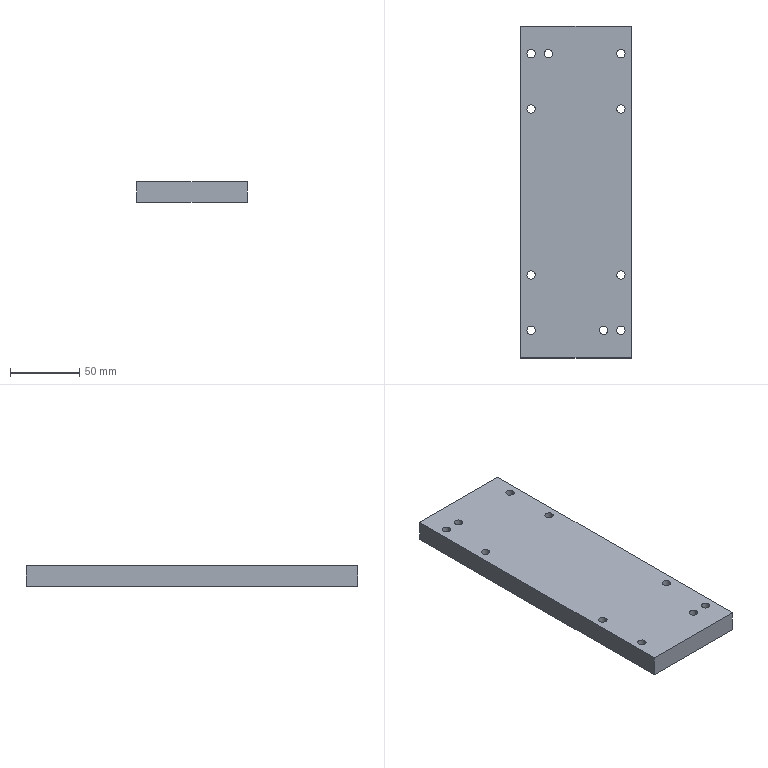Part | STEP file | SN10_008_006-02_PLACA | 1 solid | 16 faces | box 80 x 240 x 15 mm | volume 283759 mm3 | cylinder 10 | plane 6 | commonest cylinder face diameters 6 x10
STEP:
#1=CARTESIAN_POINT('',(0.,0.,0.));
#2=DIRECTION('',(0.,0.,1.));
#3=DIRECTION('',(1.,0.,0.));
#4=AXIS2_PLACEMENT_3D('',#1,#2,#3);
#5=CARTESIAN_POINT('',(323.629,430.,-115.));
#6=VERTEX_POINT('',#5);
#7=CARTESIAN_POINT('',(323.629,190.,-115.));
#8=VERTEX_POINT('',#7);
#9=CARTESIAN_POINT('',(323.629,430.,-115.));
#10=DIRECTION('',(0.,-1.,0.));
#11=VECTOR('',#10,1.);
#12=LINE('',#9,#11);
#13=CARTESIAN_POINT('',(0.,0.,-115.));
#14=DIRECTION('',(0.,0.,1.));
#15=DIRECTION('',(1.,0.,0.));
#16=AXIS2_PLACEMENT_3D('',#13,#14,#15);
#17=PLANE('',#16);
#18=CARTESIAN_POINT('',(323.629,430.));
#19=DIRECTION('',(0.,-1.));
#20=VECTOR('',#19,1.);
#21=LINE('',#18,#20);
#22=(GEOMETRIC_REPRESENTATION_CONTEXT(2)PARAMETRIC_REPRESENTATION_CONTEXT()REPRESENTATION_CONTEXT('',''));
#23=DEFINITIONAL_REPRESENTATION('',(#21),#22);
#24=PCURVE('',#17,#23);
#25=CARTESIAN_POINT('',(323.629,430.,-115.));
#26=DIRECTION('',(-1.,0.,0.));
#27=DIRECTION('',(0.,0.,1.));
#28=AXIS2_PLACEMENT_3D('',#25,#26,#27);
#29=PLANE('',#28);
#30=CARTESIAN_POINT('',(0.,0.));
#31=DIRECTION('',(0.,-1.));
#32=VECTOR('',#31,1.);
#33=LINE('',#30,#32);
#34=(GEOMETRIC_REPRESENTATION_CONTEXT(2)PARAMETRIC_REPRESENTATION_CONTEXT()REPRESENTATION_CONTEXT('',''));
#35=DEFINITIONAL_REPRESENTATION('',(#33),#34);
#36=PCURVE('',#29,#35);
#37=SURFACE_CURVE('',#12,(#24,#36),.PCURVE_S1.);
#38=EDGE_CURVE('',#6,#8,#37,.T.);
#39=ORIENTED_EDGE('',*,*,#38,.T.);
#40=CARTESIAN_POINT('',(243.629,190.,-115.));
#41=VERTEX_POINT('',#40);
#42=CARTESIAN_POINT('',(323.629,190.,-115.));
#43=DIRECTION('',(-1.,0.,0.));
#44=VECTOR('',#43,1.);
#45=LINE('',#42,#44);
#46=CARTESIAN_POINT('',(323.629,190.));
#47=DIRECTION('',(-1.,0.));
#48=VECTOR('',#47,1.);
#49=LINE('',#46,#48);
#50=(GEOMETRIC_REPRESENTATION_CONTEXT(2)PARAMETRIC_REPRESENTATION_CONTEXT()REPRESENTATION_CONTEXT('',''));
#51=DEFINITIONAL_REPRESENTATION('',(#49),#50);
#52=PCURVE('',#17,#51);
#53=CARTESIAN_POINT('',(323.629,190.,-115.));
#54=DIRECTION('',(0.,1.,0.));
#55=DIRECTION('',(0.,0.,1.));
#56=AXIS2_PLACEMENT_3D('',#53,#54,#55);
#57=PLANE('',#56);
#58=CARTESIAN_POINT('',(0.,0.));
#59=DIRECTION('',(0.,-1.));
#60=VECTOR('',#59,1.);
#61=LINE('',#58,#60);
#62=(GEOMETRIC_REPRESENTATION_CONTEXT(2)PARAMETRIC_REPRESENTATION_CONTEXT()REPRESENTATION_CONTEXT('',''));
#63=DEFINITIONAL_REPRESENTATION('',(#61),#62);
#64=PCURVE('',#57,#63);
#65=SURFACE_CURVE('',#45,(#52,#64),.PCURVE_S1.);
#66=EDGE_CURVE('',#8,#41,#65,.T.);
#67=ORIENTED_EDGE('',*,*,#66,.T.);
#68=CARTESIAN_POINT('',(243.629,430.,-115.));
#69=VERTEX_POINT('',#68);
#70=CARTESIAN_POINT('',(243.629,190.,-115.));
#71=DIRECTION('',(0.,1.,0.));
#72=VECTOR('',#71,1.);
#73=LINE('',#70,#72);
#74=CARTESIAN_POINT('',(243.629,190.));
#75=DIRECTION('',(0.,1.));
#76=VECTOR('',#75,1.);
#77=LINE('',#74,#76);
#78=(GEOMETRIC_REPRESENTATION_CONTEXT(2)PARAMETRIC_REPRESENTATION_CONTEXT()REPRESENTATION_CONTEXT('',''));
#79=DEFINITIONAL_REPRESENTATION('',(#77),#78);
#80=PCURVE('',#17,#79);
#81=CARTESIAN_POINT('',(243.629,190.,-115.));
#82=DIRECTION('',(1.,0.,0.));
#83=DIRECTION('',(0.,0.,-1.));
#84=AXIS2_PLACEMENT_3D('',#81,#82,#83);
#85=PLANE('',#84);
#86=CARTESIAN_POINT('',(0.,0.));
#87=DIRECTION('',(0.,1.));
#88=VECTOR('',#87,1.);
#89=LINE('',#86,#88);
#90=(GEOMETRIC_REPRESENTATION_CONTEXT(2)PARAMETRIC_REPRESENTATION_CONTEXT()REPRESENTATION_CONTEXT('',''));
#91=DEFINITIONAL_REPRESENTATION('',(#89),#90);
#92=PCURVE('',#85,#91);
#93=SURFACE_CURVE('',#73,(#80,#92),.PCURVE_S1.);
#94=EDGE_CURVE('',#41,#69,#93,.T.);
#95=ORIENTED_EDGE('',*,*,#94,.T.);
#96=CARTESIAN_POINT('',(243.629,430.,-115.));
#97=DIRECTION('',(1.,0.,0.));
#98=VECTOR('',#97,1.);
#99=LINE('',#96,#98);
#100=CARTESIAN_POINT('',(243.629,430.));
#101=DIRECTION('',(1.,0.));
#102=VECTOR('',#101,1.);
#103=LINE('',#100,#102);
#104=(GEOMETRIC_REPRESENTATION_CONTEXT(2)PARAMETRIC_REPRESENTATION_CONTEXT()REPRESENTATION_CONTEXT('',''));
#105=DEFINITIONAL_REPRESENTATION('',(#103),#104);
#106=PCURVE('',#17,#105);
#107=CARTESIAN_POINT('',(243.629,430.,-115.));
#108=DIRECTION('',(0.,-1.,0.));
#109=DIRECTION('',(0.,0.,-1.));
#110=AXIS2_PLACEMENT_3D('',#107,#108,#109);
#111=PLANE('',#110);
#112=CARTESIAN_POINT('',(0.,0.));
#113=DIRECTION('',(0.,1.));
#114=VECTOR('',#113,1.);
#115=LINE('',#112,#114);
#116=(GEOMETRIC_REPRESENTATION_CONTEXT(2)PARAMETRIC_REPRESENTATION_CONTEXT()REPRESENTATION_CONTEXT('',''));
#117=DEFINITIONAL_REPRESENTATION('',(#115),#116);
#118=PCURVE('',#111,#117);
#119=SURFACE_CURVE('',#99,(#106,#118),.PCURVE_S1.);
#120=EDGE_CURVE('',#69,#6,#119,.T.);
#121=ORIENTED_EDGE('',*,*,#120,.T.);
#122=EDGE_LOOP('',(#39,#67,#95,#121));
#123=FACE_BOUND('',#122,.T.);
#124=CARTESIAN_POINT('',(318.762,211.438,-115.));
#125=VERTEX_POINT('',#124);
#126=CARTESIAN_POINT('',(316.129,210.,-115.));
#127=DIRECTION('',(0.,0.,1.));
#128=DIRECTION('',(1.,0.,0.));
#129=AXIS2_PLACEMENT_3D('',#126,#127,#128);
#130=CIRCLE('',#129,3.);
#131=CARTESIAN_POINT('',(316.129,210.));
#132=DIRECTION('',(1.,0.));
#133=AXIS2_PLACEMENT_2D('',#131,#132);
#134=CIRCLE('',#133,3.);
#135=(GEOMETRIC_REPRESENTATION_CONTEXT(2)PARAMETRIC_REPRESENTATION_CONTEXT()REPRESENTATION_CONTEXT('',''));
#136=DEFINITIONAL_REPRESENTATION('',(#134),#135);
#137=PCURVE('',#17,#136);
#138=CARTESIAN_POINT('',(316.129,210.,-114.9));
#139=DIRECTION('',(0.,0.,1.));
#140=DIRECTION('',(0.8776,0.4794,0.));
#141=AXIS2_PLACEMENT_3D('',#138,#139,#140);
#142=CYLINDRICAL_SURFACE('',#141,3.);
#143=CARTESIAN_POINT('',(-0.5,-0.1));
#144=DIRECTION('',(1.,0.));
#145=VECTOR('',#144,1.);
#146=LINE('',#143,#145);
#147=(GEOMETRIC_REPRESENTATION_CONTEXT(2)PARAMETRIC_REPRESENTATION_CONTEXT()REPRESENTATION_CONTEXT('',''));
#148=DEFINITIONAL_REPRESENTATION('',(#146),#147);
#149=PCURVE('',#142,#148);
#150=SURFACE_CURVE('',#130,(#137,#149),.PCURVE_S1.);
#151=EDGE_CURVE('',#125,#125,#150,.T.);
#152=ORIENTED_EDGE('',*,*,#151,.T.);
#153=EDGE_LOOP('',(#152));
#154=FACE_BOUND('',#153,.T.);
#155=CARTESIAN_POINT('',(253.762,411.438,-115.));
#156=VERTEX_POINT('',#155);
#157=CARTESIAN_POINT('',(251.129,410.,-115.));
#158=DIRECTION('',(0.,0.,1.));
#159=DIRECTION('',(1.,0.,0.));
#160=AXIS2_PLACEMENT_3D('',#157,#158,#159);
#161=CIRCLE('',#160,3.);
#162=CARTESIAN_POINT('',(251.129,410.));
#163=DIRECTION('',(1.,0.));
#164=AXIS2_PLACEMENT_2D('',#162,#163);
#165=CIRCLE('',#164,3.);
#166=(GEOMETRIC_REPRESENTATION_CONTEXT(2)PARAMETRIC_REPRESENTATION_CONTEXT()REPRESENTATION_CONTEXT('',''));
#167=DEFINITIONAL_REPRESENTATION('',(#165),#166);
#168=PCURVE('',#17,#167);
#169=CARTESIAN_POINT('',(251.129,410.,-114.9));
#170=DIRECTION('',(0.,0.,1.));
#171=DIRECTION('',(0.8776,0.4794,0.));
#172=AXIS2_PLACEMENT_3D('',#169,#170,#171);
#173=CYLINDRICAL_SURFACE('',#172,3.);
#174=CARTESIAN_POINT('',(-0.5,-0.1));
#175=DIRECTION('',(1.,0.));
#176=VECTOR('',#175,1.);
#177=LINE('',#174,#176);
#178=(GEOMETRIC_REPRESENTATION_CONTEXT(2)PARAMETRIC_REPRESENTATION_CONTEXT()REPRESENTATION_CONTEXT('',''));
#179=DEFINITIONAL_REPRESENTATION('',(#177),#178);
#180=PCURVE('',#173,#179);
#181=SURFACE_CURVE('',#161,(#168,#180),.PCURVE_S1.);
#182=EDGE_CURVE('',#156,#156,#181,.T.);
#183=ORIENTED_EDGE('',*,*,#182,.T.);
#184=EDGE_LOOP('',(#183));
#185=FACE_BOUND('',#184,.T.);
#186=CARTESIAN_POINT('',(306.262,211.438,-115.));
#187=VERTEX_POINT('',#186);
#188=CARTESIAN_POINT('',(303.629,210.,-115.));
#189=DIRECTION('',(0.,0.,1.));
#190=DIRECTION('',(1.,0.,0.));
#191=AXIS2_PLACEMENT_3D('',#188,#189,#190);
#192=CIRCLE('',#191,3.);
#193=CARTESIAN_POINT('',(303.629,210.));
#194=DIRECTION('',(1.,0.));
#195=AXIS2_PLACEMENT_2D('',#193,#194);
#196=CIRCLE('',#195,3.);
#197=(GEOMETRIC_REPRESENTATION_CONTEXT(2)PARAMETRIC_REPRESENTATION_CONTEXT()REPRESENTATION_CONTEXT('',''));
#198=DEFINITIONAL_REPRESENTATION('',(#196),#197);
#199=PCURVE('',#17,#198);
#200=CARTESIAN_POINT('',(303.629,210.,-114.9));
#201=DIRECTION('',(0.,0.,1.));
#202=DIRECTION('',(0.8776,0.4794,0.));
#203=AXIS2_PLACEMENT_3D('',#200,#201,#202);
#204=CYLINDRICAL_SURFACE('',#203,3.);
#205=CARTESIAN_POINT('',(-0.5,-0.1));
#206=DIRECTION('',(1.,0.));
#207=VECTOR('',#206,1.);
#208=LINE('',#205,#207);
#209=(GEOMETRIC_REPRESENTATION_CONTEXT(2)PARAMETRIC_REPRESENTATION_CONTEXT()REPRESENTATION_CONTEXT('',''));
#210=DEFINITIONAL_REPRESENTATION('',(#208),#209);
#211=PCURVE('',#204,#210);
#212=SURFACE_CURVE('',#192,(#199,#211),.PCURVE_S1.);
#213=EDGE_CURVE('',#187,#187,#212,.T.);
#214=ORIENTED_EDGE('',*,*,#213,.T.);
#215=EDGE_LOOP('',(#214));
#216=FACE_BOUND('',#215,.T.);
#217=CARTESIAN_POINT('',(266.262,411.438,-115.));
#218=VERTEX_POINT('',#217);
#219=CARTESIAN_POINT('',(263.629,410.,-115.));
#220=DIRECTION('',(0.,0.,1.));
#221=DIRECTION('',(1.,0.,0.));
#222=AXIS2_PLACEMENT_3D('',#219,#220,#221);
#223=CIRCLE('',#222,3.);
#224=CARTESIAN_POINT('',(263.629,410.));
#225=DIRECTION('',(1.,0.));
#226=AXIS2_PLACEMENT_2D('',#224,#225);
#227=CIRCLE('',#226,3.);
#228=(GEOMETRIC_REPRESENTATION_CONTEXT(2)PARAMETRIC_REPRESENTATION_CONTEXT()REPRESENTATION_CONTEXT('',''));
#229=DEFINITIONAL_REPRESENTATION('',(#227),#228);
#230=PCURVE('',#17,#229);
#231=CARTESIAN_POINT('',(263.629,410.,-114.9));
#232=DIRECTION('',(0.,0.,1.));
#233=DIRECTION('',(0.8776,0.4794,0.));
#234=AXIS2_PLACEMENT_3D('',#231,#232,#233);
#235=CYLINDRICAL_SURFACE('',#234,3.);
#236=CARTESIAN_POINT('',(-0.5,-0.1));
#237=DIRECTION('',(1.,0.));
#238=VECTOR('',#237,1.);
#239=LINE('',#236,#238);
#240=(GEOMETRIC_REPRESENTATION_CONTEXT(2)PARAMETRIC_REPRESENTATION_CONTEXT()REPRESENTATION_CONTEXT('',''));
#241=DEFINITIONAL_REPRESENTATION('',(#239),#240);
#242=PCURVE('',#235,#241);
#243=SURFACE_CURVE('',#223,(#230,#242),.PCURVE_S1.);
#244=EDGE_CURVE('',#218,#218,#243,.T.);
#245=ORIENTED_EDGE('',*,*,#244,.T.);
#246=EDGE_LOOP('',(#245));
#247=FACE_BOUND('',#246,.T.);
#248=CARTESIAN_POINT('',(313.496,408.562,-115.));
#249=VERTEX_POINT('',#248);
#250=CARTESIAN_POINT('',(316.129,410.,-115.));
#251=DIRECTION('',(0.,0.,1.));
#252=DIRECTION('',(1.,0.,0.));
#253=AXIS2_PLACEMENT_3D('',#250,#251,#252);
#254=CIRCLE('',#253,3.);
#255=CARTESIAN_POINT('',(316.129,410.));
#256=DIRECTION('',(1.,0.));
#257=AXIS2_PLACEMENT_2D('',#255,#256);
#258=CIRCLE('',#257,3.);
#259=(GEOMETRIC_REPRESENTATION_CONTEXT(2)PARAMETRIC_REPRESENTATION_CONTEXT()REPRESENTATION_CONTEXT('',''));
#260=DEFINITIONAL_REPRESENTATION('',(#258),#259);
#261=PCURVE('',#17,#260);
#262=CARTESIAN_POINT('',(316.129,410.,-114.9));
#263=DIRECTION('',(0.,0.,1.));
#264=DIRECTION('',(0.8776,0.4794,0.));
#265=AXIS2_PLACEMENT_3D('',#262,#263,#264);
#266=CYLINDRICAL_SURFACE('',#265,3.);
#267=CARTESIAN_POINT('',(-0.5,-0.1));
#268=DIRECTION('',(1.,0.));
#269=VECTOR('',#268,1.);
#270=LINE('',#267,#269);
#271=(GEOMETRIC_REPRESENTATION_CONTEXT(2)PARAMETRIC_REPRESENTATION_CONTEXT()REPRESENTATION_CONTEXT('',''));
#272=DEFINITIONAL_REPRESENTATION('',(#270),#271);
#273=PCURVE('',#266,#272);
#274=SURFACE_CURVE('',#254,(#261,#273),.PCURVE_S1.);
#275=EDGE_CURVE('',#249,#249,#274,.T.);
#276=ORIENTED_EDGE('',*,*,#275,.T.);
#277=EDGE_LOOP('',(#276));
#278=FACE_BOUND('',#277,.T.);
#279=CARTESIAN_POINT('',(248.496,368.562,-115.));
#280=VERTEX_POINT('',#279);
#281=CARTESIAN_POINT('',(251.129,370.,-115.));
#282=DIRECTION('',(0.,0.,1.));
#283=DIRECTION('',(1.,0.,0.));
#284=AXIS2_PLACEMENT_3D('',#281,#282,#283);
#285=CIRCLE('',#284,3.);
#286=CARTESIAN_POINT('',(251.129,370.));
#287=DIRECTION('',(1.,0.));
#288=AXIS2_PLACEMENT_2D('',#286,#287);
#289=CIRCLE('',#288,3.);
#290=(GEOMETRIC_REPRESENTATION_CONTEXT(2)PARAMETRIC_REPRESENTATION_CONTEXT()REPRESENTATION_CONTEXT('',''));
#291=DEFINITIONAL_REPRESENTATION('',(#289),#290);
#292=PCURVE('',#17,#291);
#293=CARTESIAN_POINT('',(251.129,370.,-114.9));
#294=DIRECTION('',(0.,0.,1.));
#295=DIRECTION('',(0.8776,0.4794,0.));
#296=AXIS2_PLACEMENT_3D('',#293,#294,#295);
#297=CYLINDRICAL_SURFACE('',#296,3.);
#298=CARTESIAN_POINT('',(-0.5,-0.1));
#299=DIRECTION('',(1.,0.));
#300=VECTOR('',#299,1.);
#301=LINE('',#298,#300);
#302=(GEOMETRIC_REPRESENTATION_CONTEXT(2)PARAMETRIC_REPRESENTATION_CONTEXT()REPRESENTATION_CONTEXT('',''));
#303=DEFINITIONAL_REPRESENTATION('',(#301),#302);
#304=PCURVE('',#297,#303);
#305=SURFACE_CURVE('',#285,(#292,#304),.PCURVE_S1.);
#306=EDGE_CURVE('',#280,#280,#305,.T.);
#307=ORIENTED_EDGE('',*,*,#306,.T.);
#308=EDGE_LOOP('',(#307));
#309=FACE_BOUND('',#308,.T.);
#310=CARTESIAN_POINT('',(313.496,368.562,-115.));
#311=VERTEX_POINT('',#310);
#312=CARTESIAN_POINT('',(316.129,370.,-115.));
#313=DIRECTION('',(0.,0.,1.));
#314=DIRECTION('',(1.,0.,0.));
#315=AXIS2_PLACEMENT_3D('',#312,#313,#314);
#316=CIRCLE('',#315,3.);
#317=CARTESIAN_POINT('',(316.129,370.));
#318=DIRECTION('',(1.,0.));
#319=AXIS2_PLACEMENT_2D('',#317,#318);
#320=CIRCLE('',#319,3.);
#321=(GEOMETRIC_REPRESENTATION_CONTEXT(2)PARAMETRIC_REPRESENTATION_CONTEXT()REPRESENTATION_CONTEXT('',''));
#322=DEFINITIONAL_REPRESENTATION('',(#320),#321);
#323=PCURVE('',#17,#322);
#324=CARTESIAN_POINT('',(316.129,370.,-114.9));
#325=DIRECTION('',(0.,0.,1.));
#326=DIRECTION('',(0.8776,0.4794,0.));
#327=AXIS2_PLACEMENT_3D('',#324,#325,#326);
#328=CYLINDRICAL_SURFACE('',#327,3.);
#329=CARTESIAN_POINT('',(-0.5,-0.1));
#330=DIRECTION('',(1.,0.));
#331=VECTOR('',#330,1.);
#332=LINE('',#329,#331);
#333=(GEOMETRIC_REPRESENTATION_CONTEXT(2)PARAMETRIC_REPRESENTATION_CONTEXT()REPRESENTATION_CONTEXT('',''));
#334=DEFINITIONAL_REPRESENTATION('',(#332),#333);
#335=PCURVE('',#328,#334);
#336=SURFACE_CURVE('',#316,(#323,#335),.PCURVE_S1.);
#337=EDGE_CURVE('',#311,#311,#336,.T.);
#338=ORIENTED_EDGE('',*,*,#337,.T.);
#339=EDGE_LOOP('',(#338));
#340=FACE_BOUND('',#339,.T.);
#341=CARTESIAN_POINT('',(253.762,211.438,-115.));
#342=VERTEX_POINT('',#341);
#343=CARTESIAN_POINT('',(251.129,210.,-115.));
#344=DIRECTION('',(0.,0.,1.));
#345=DIRECTION('',(1.,0.,0.));
#346=AXIS2_PLACEMENT_3D('',#343,#344,#345);
#347=CIRCLE('',#346,3.);
#348=CARTESIAN_POINT('',(251.129,210.));
#349=DIRECTION('',(1.,0.));
#350=AXIS2_PLACEMENT_2D('',#348,#349);
#351=CIRCLE('',#350,3.);
#352=(GEOMETRIC_REPRESENTATION_CONTEXT(2)PARAMETRIC_REPRESENTATION_CONTEXT()REPRESENTATION_CONTEXT('',''));
#353=DEFINITIONAL_REPRESENTATION('',(#351),#352);
#354=PCURVE('',#17,#353);
#355=CARTESIAN_POINT('',(251.129,210.,-114.9));
#356=DIRECTION('',(0.,0.,1.));
#357=DIRECTION('',(0.8776,0.4794,0.));
#358=AXIS2_PLACEMENT_3D('',#355,#356,#357);
#359=CYLINDRICAL_SURFACE('',#358,3.);
#360=CARTESIAN_POINT('',(-0.5,-0.1));
#361=DIRECTION('',(1.,0.));
#362=VECTOR('',#361,1.);
#363=LINE('',#360,#362);
#364=(GEOMETRIC_REPRESENTATION_CONTEXT(2)PARAMETRIC_REPRESENTATION_CONTEXT()REPRESENTATION_CONTEXT('',''));
#365=DEFINITIONAL_REPRESENTATION('',(#363),#364);
#366=PCURVE('',#359,#365);
#367=SURFACE_CURVE('',#347,(#354,#366),.PCURVE_S1.);
#368=EDGE_CURVE('',#342,#342,#367,.T.);
#369=ORIENTED_EDGE('',*,*,#368,.T.);
#370=EDGE_LOOP('',(#369));
#371=FACE_BOUND('',#370,.T.);
#372=CARTESIAN_POINT('',(318.762,251.438,-115.));
#373=VERTEX_POINT('',#372);
#374=CARTESIAN_POINT('',(316.129,250.,-115.));
#375=DIRECTION('',(0.,0.,1.));
#376=DIRECTION('',(1.,0.,0.));
#377=AXIS2_PLACEMENT_3D('',#374,#375,#376);
#378=CIRCLE('',#377,3.);
#379=CARTESIAN_POINT('',(316.129,250.));
#380=DIRECTION('',(1.,0.));
#381=AXIS2_PLACEMENT_2D('',#379,#380);
#382=CIRCLE('',#381,3.);
#383=(GEOMETRIC_REPRESENTATION_CONTEXT(2)PARAMETRIC_REPRESENTATION_CONTEXT()REPRESENTATION_CONTEXT('',''));
#384=DEFINITIONAL_REPRESENTATION('',(#382),#383);
#385=PCURVE('',#17,#384);
#386=CARTESIAN_POINT('',(316.129,250.,-114.9));
#387=DIRECTION('',(0.,0.,1.));
#388=DIRECTION('',(0.8776,0.4794,0.));
#389=AXIS2_PLACEMENT_3D('',#386,#387,#388);
#390=CYLINDRICAL_SURFACE('',#389,3.);
#391=CARTESIAN_POINT('',(-0.5,-0.1));
#392=DIRECTION('',(1.,0.));
#393=VECTOR('',#392,1.);
#394=LINE('',#391,#393);
#395=(GEOMETRIC_REPRESENTATION_CONTEXT(2)PARAMETRIC_REPRESENTATION_CONTEXT()REPRESENTATION_CONTEXT('',''));
#396=DEFINITIONAL_REPRESENTATION('',(#394),#395);
#397=PCURVE('',#390,#396);
#398=SURFACE_CURVE('',#378,(#385,#397),.PCURVE_S1.);
#399=EDGE_CURVE('',#373,#373,#398,.T.);
#400=ORIENTED_EDGE('',*,*,#399,.T.);
#401=EDGE_LOOP('',(#400));
#402=FACE_BOUND('',#401,.T.);
#403=CARTESIAN_POINT('',(253.762,251.438,-115.));
#404=VERTEX_POINT('',#403);
#405=CARTESIAN_POINT('',(251.129,250.,-115.));
#406=DIRECTION('',(0.,0.,1.));
#407=DIRECTION('',(1.,0.,0.));
#408=AXIS2_PLACEMENT_3D('',#405,#406,#407);
#409=CIRCLE('',#408,3.);
#410=CARTESIAN_POINT('',(251.129,250.));
#411=DIRECTION('',(1.,0.));
#412=AXIS2_PLACEMENT_2D('',#410,#411);
#413=CIRCLE('',#412,3.);
#414=(GEOMETRIC_REPRESENTATION_CONTEXT(2)PARAMETRIC_REPRESENTATION_CONTEXT()REPRESENTATION_CONTEXT('',''));
#415=DEFINITIONAL_REPRESENTATION('',(#413),#414);
#416=PCURVE('',#17,#415);
#417=CARTESIAN_POINT('',(251.129,250.,-114.9));
#418=DIRECTION('',(0.,0.,1.));
#419=DIRECTION('',(0.8776,0.4794,0.));
#420=AXIS2_PLACEMENT_3D('',#417,#418,#419);
#421=CYLINDRICAL_SURFACE('',#420,3.);
#422=CARTESIAN_POINT('',(-0.5,-0.1));
#423=DIRECTION('',(1.,0.));
#424=VECTOR('',#423,1.);
#425=LINE('',#422,#424);
#426=(GEOMETRIC_REPRESENTATION_CONTEXT(2)PARAMETRIC_REPRESENTATION_CONTEXT()REPRESENTATION_CONTEXT('',''));
#427=DEFINITIONAL_REPRESENTATION('',(#425),#426);
#428=PCURVE('',#421,#427);
#429=SURFACE_CURVE('',#409,(#416,#428),.PCURVE_S1.);
#430=EDGE_CURVE('',#404,#404,#429,.T.);
#431=ORIENTED_EDGE('',*,*,#430,.T.);
#432=EDGE_LOOP('',(#431));
#433=FACE_BOUND('',#432,.T.);
#434=ADVANCED_FACE('',(#123,#154,#185,#216,#247,#278,#309,#340,#371,#402,#433),#17,.F.);
#435=CARTESIAN_POINT('',(253.762,211.438,-100.));
#436=VERTEX_POINT('',#435);
#437=CARTESIAN_POINT('',(251.129,210.,-100.));
#438=DIRECTION('',(0.,0.,1.));
#439=DIRECTION('',(1.,0.,0.));
#440=AXIS2_PLACEMENT_3D('',#437,#438,#439);
#441=CIRCLE('',#440,3.);
#442=CARTESIAN_POINT('',(-0.5,14.9));
#443=DIRECTION('',(1.,0.));
#444=VECTOR('',#443,1.);
#445=LINE('',#442,#444);
#446=(GEOMETRIC_REPRESENTATION_CONTEXT(2)PARAMETRIC_REPRESENTATION_CONTEXT()REPRESENTATION_CONTEXT('',''));
#447=DEFINITIONAL_REPRESENTATION('',(#445),#446);
#448=PCURVE('',#359,#447);
#449=CARTESIAN_POINT('',(0.,0.,-100.));
#450=DIRECTION('',(0.,0.,1.));
#451=DIRECTION('',(1.,0.,0.));
#452=AXIS2_PLACEMENT_3D('',#449,#450,#451);
#453=PLANE('',#452);
#454=CARTESIAN_POINT('',(251.129,210.));
#455=DIRECTION('',(1.,0.));
#456=AXIS2_PLACEMENT_2D('',#454,#455);
#457=CIRCLE('',#456,3.);
#458=(GEOMETRIC_REPRESENTATION_CONTEXT(2)PARAMETRIC_REPRESENTATION_CONTEXT()REPRESENTATION_CONTEXT('',''));
#459=DEFINITIONAL_REPRESENTATION('',(#457),#458);
#460=PCURVE('',#453,#459);
#461=SURFACE_CURVE('',#441,(#448,#460),.PCURVE_S1.);
#462=EDGE_CURVE('',#436,#436,#461,.T.);
#463=ORIENTED_EDGE('',*,*,#462,.F.);
#464=CARTESIAN_POINT('',(253.762,211.438,-115.));
#465=CARTESIAN_POINT('',(253.762,211.438,-100.));
#466=B_SPLINE_CURVE_WITH_KNOTS('',1,(#464,#465),.UNSPECIFIED.,.F.,.F.,(2,2),(-0.1,14.9),.PIECEWISE_BEZIER_KNOTS.);
#467=CARTESIAN_POINT('',(0.,0.));
#468=DIRECTION('',(0.,1.));
#469=VECTOR('',#468,1.);
#470=LINE('',#467,#469);
#471=(GEOMETRIC_REPRESENTATION_CONTEXT(2)PARAMETRIC_REPRESENTATION_CONTEXT()REPRESENTATION_CONTEXT('',''));
#472=DEFINITIONAL_REPRESENTATION('',(#470),#471);
#473=PCURVE('',#359,#472);
#474=CARTESIAN_POINT('',(6.283,0.));
#475=DIRECTION('',(0.,1.));
#476=VECTOR('',#475,1.);
#477=LINE('',#474,#476);
#478=(GEOMETRIC_REPRESENTATION_CONTEXT(2)PARAMETRIC_REPRESENTATION_CONTEXT()REPRESENTATION_CONTEXT('',''));
#479=DEFINITIONAL_REPRESENTATION('',(#477),#478);
#480=PCURVE('',#359,#479);
#481=SEAM_CURVE('',#466,(#473,#480),.PCURVE_S1.);
#482=EDGE_CURVE('',#342,#436,#481,.T.);
#483=ORIENTED_EDGE('',*,*,#482,.F.);
#484=ORIENTED_EDGE('',*,*,#368,.T.);
#485=ORIENTED_EDGE('',*,*,#482,.T.);
#486=EDGE_LOOP('',(#463,#483,#484,#485));
#487=FACE_BOUND('',#486,.F.);
#488=ADVANCED_FACE('',(#487),#359,.F.);
#489=CARTESIAN_POINT('',(318.762,251.438,-100.));
#490=VERTEX_POINT('',#489);
#491=CARTESIAN_POINT('',(316.129,250.,-100.));
#492=DIRECTION('',(0.,0.,1.));
#493=DIRECTION('',(1.,0.,0.));
#494=AXIS2_PLACEMENT_3D('',#491,#492,#493);
#495=CIRCLE('',#494,3.);
#496=CARTESIAN_POINT('',(-0.5,14.9));
#497=DIRECTION('',(1.,0.));
#498=VECTOR('',#497,1.);
#499=LINE('',#496,#498);
#500=(GEOMETRIC_REPRESENTATION_CONTEXT(2)PARAMETRIC_REPRESENTATION_CONTEXT()REPRESENTATION_CONTEXT('',''));
#501=DEFINITIONAL_REPRESENTATION('',(#499),#500);
#502=PCURVE('',#390,#501);
#503=CARTESIAN_POINT('',(316.129,250.));
#504=DIRECTION('',(1.,0.));
#505=AXIS2_PLACEMENT_2D('',#503,#504);
#506=CIRCLE('',#505,3.);
#507=(GEOMETRIC_REPRESENTATION_CONTEXT(2)PARAMETRIC_REPRESENTATION_CONTEXT()REPRESENTATION_CONTEXT('',''));
#508=DEFINITIONAL_REPRESENTATION('',(#506),#507);
#509=PCURVE('',#453,#508);
#510=SURFACE_CURVE('',#495,(#502,#509),.PCURVE_S1.);
#511=EDGE_CURVE('',#490,#490,#510,.T.);
#512=ORIENTED_EDGE('',*,*,#511,.F.);
#513=CARTESIAN_POINT('',(318.762,251.438,-115.));
#514=CARTESIAN_POINT('',(318.762,251.438,-100.));
#515=B_SPLINE_CURVE_WITH_KNOTS('',1,(#513,#514),.UNSPECIFIED.,.F.,.F.,(2,2),(-0.1,14.9),.PIECEWISE_BEZIER_KNOTS.);
#516=CARTESIAN_POINT('',(0.,0.));
#517=DIRECTION('',(0.,1.));
#518=VECTOR('',#517,1.);
#519=LINE('',#516,#518);
#520=(GEOMETRIC_REPRESENTATION_CONTEXT(2)PARAMETRIC_REPRESENTATION_CONTEXT()REPRESENTATION_CONTEXT('',''));
#521=DEFINITIONAL_REPRESENTATION('',(#519),#520);
#522=PCURVE('',#390,#521);
#523=CARTESIAN_POINT('',(6.283,0.));
#524=DIRECTION('',(0.,1.));
#525=VECTOR('',#524,1.);
#526=LINE('',#523,#525);
#527=(GEOMETRIC_REPRESENTATION_CONTEXT(2)PARAMETRIC_REPRESENTATION_CONTEXT()REPRESENTATION_CONTEXT('',''));
#528=DEFINITIONAL_REPRESENTATION('',(#526),#527);
#529=PCURVE('',#390,#528);
#530=SEAM_CURVE('',#515,(#522,#529),.PCURVE_S1.);
#531=EDGE_CURVE('',#373,#490,#530,.T.);
#532=ORIENTED_EDGE('',*,*,#531,.F.);
#533=ORIENTED_EDGE('',*,*,#399,.T.);
#534=ORIENTED_EDGE('',*,*,#531,.T.);
#535=EDGE_LOOP('',(#512,#532,#533,#534));
#536=FACE_BOUND('',#535,.F.);
#537=ADVANCED_FACE('',(#536),#390,.F.);
#538=CARTESIAN_POINT('',(253.762,251.438,-100.));
#539=VERTEX_POINT('',#538);
#540=CARTESIAN_POINT('',(251.129,250.,-100.));
#541=DIRECTION('',(0.,0.,1.));
#542=DIRECTION('',(1.,0.,0.));
#543=AXIS2_PLACEMENT_3D('',#540,#541,#542);
#544=CIRCLE('',#543,3.);
#545=CARTESIAN_POINT('',(-0.5,14.9));
#546=DIRECTION('',(1.,0.));
#547=VECTOR('',#546,1.);
#548=LINE('',#545,#547);
#549=(GEOMETRIC_REPRESENTATION_CONTEXT(2)PARAMETRIC_REPRESENTATION_CONTEXT()REPRESENTATION_CONTEXT('',''));
#550=DEFINITIONAL_REPRESENTATION('',(#548),#549);
#551=PCURVE('',#421,#550);
#552=CARTESIAN_POINT('',(251.129,250.));
#553=DIRECTION('',(1.,0.));
#554=AXIS2_PLACEMENT_2D('',#552,#553);
#555=CIRCLE('',#554,3.);
#556=(GEOMETRIC_REPRESENTATION_CONTEXT(2)PARAMETRIC_REPRESENTATION_CONTEXT()REPRESENTATION_CONTEXT('',''));
#557=DEFINITIONAL_REPRESENTATION('',(#555),#556);
#558=PCURVE('',#453,#557);
#559=SURFACE_CURVE('',#544,(#551,#558),.PCURVE_S1.);
#560=EDGE_CURVE('',#539,#539,#559,.T.);
#561=ORIENTED_EDGE('',*,*,#560,.F.);
#562=CARTESIAN_POINT('',(253.762,251.438,-115.));
#563=CARTESIAN_POINT('',(253.762,251.438,-100.));
#564=B_SPLINE_CURVE_WITH_KNOTS('',1,(#562,#563),.UNSPECIFIED.,.F.,.F.,(2,2),(-0.1,14.9),.PIECEWISE_BEZIER_KNOTS.);
#565=CARTESIAN_POINT('',(0.,0.));
#566=DIRECTION('',(0.,1.));
#567=VECTOR('',#566,1.);
#568=LINE('',#565,#567);
#569=(GEOMETRIC_REPRESENTATION_CONTEXT(2)PARAMETRIC_REPRESENTATION_CONTEXT()REPRESENTATION_CONTEXT('',''));
#570=DEFINITIONAL_REPRESENTATION('',(#568),#569);
#571=PCURVE('',#421,#570);
#572=CARTESIAN_POINT('',(6.283,0.));
#573=DIRECTION('',(0.,1.));
#574=VECTOR('',#573,1.);
#575=LINE('',#572,#574);
#576=(GEOMETRIC_REPRESENTATION_CONTEXT(2)PARAMETRIC_REPRESENTATION_CONTEXT()REPRESENTATION_CONTEXT('',''));
#577=DEFINITIONAL_REPRESENTATION('',(#575),#576);
#578=PCURVE('',#421,#577);
#579=SEAM_CURVE('',#564,(#571,#578),.PCURVE_S1.);
#580=EDGE_CURVE('',#404,#539,#579,.T.);
#581=ORIENTED_EDGE('',*,*,#580,.F.);
#582=ORIENTED_EDGE('',*,*,#430,.T.);
#583=ORIENTED_EDGE('',*,*,#580,.T.);
#584=EDGE_LOOP('',(#561,#581,#582,#583));
#585=FACE_BOUND('',#584,.F.);
#586=ADVANCED_FACE('',(#585),#421,.F.);
#587=CARTESIAN_POINT('',(253.762,411.438,-100.));
#588=VERTEX_POINT('',#587);
#589=CARTESIAN_POINT('',(251.129,410.,-100.));
#590=DIRECTION('',(0.,0.,1.));
#591=DIRECTION('',(1.,0.,0.));
#592=AXIS2_PLACEMENT_3D('',#589,#590,#591);
#593=CIRCLE('',#592,3.);
#594=CARTESIAN_POINT('',(-0.5,14.9));
#595=DIRECTION('',(1.,0.));
#596=VECTOR('',#595,1.);
#597=LINE('',#594,#596);
#598=(GEOMETRIC_REPRESENTATION_CONTEXT(2)PARAMETRIC_REPRESENTATION_CONTEXT()REPRESENTATION_CONTEXT('',''));
#599=DEFINITIONAL_REPRESENTATION('',(#597),#598);
#600=PCURVE('',#173,#599);
#601=CARTESIAN_POINT('',(251.129,410.));
#602=DIRECTION('',(1.,0.));
#603=AXIS2_PLACEMENT_2D('',#601,#602);
#604=CIRCLE('',#603,3.);
#605=(GEOMETRIC_REPRESENTATION_CONTEXT(2)PARAMETRIC_REPRESENTATION_CONTEXT()REPRESENTATION_CONTEXT('',''));
#606=DEFINITIONAL_REPRESENTATION('',(#604),#605);
#607=PCURVE('',#453,#606);
#608=SURFACE_CURVE('',#593,(#600,#607),.PCURVE_S1.);
#609=EDGE_CURVE('',#588,#588,#608,.T.);
#610=ORIENTED_EDGE('',*,*,#609,.F.);
#611=CARTESIAN_POINT('',(253.762,411.438,-115.));
#612=CARTESIAN_POINT('',(253.762,411.438,-100.));
#613=B_SPLINE_CURVE_WITH_KNOTS('',1,(#611,#612),.UNSPECIFIED.,.F.,.F.,(2,2),(-0.1,14.9),.PIECEWISE_BEZIER_KNOTS.);
#614=CARTESIAN_POINT('',(0.,0.));
#615=DIRECTION('',(0.,1.));
#616=VECTOR('',#615,1.);
#617=LINE('',#614,#616);
#618=(GEOMETRIC_REPRESENTATION_CONTEXT(2)PARAMETRIC_REPRESENTATION_CONTEXT()REPRESENTATION_CONTEXT('',''));
#619=DEFINITIONAL_REPRESENTATION('',(#617),#618);
#620=PCURVE('',#173,#619);
#621=CARTESIAN_POINT('',(6.283,0.));
#622=DIRECTION('',(0.,1.));
#623=VECTOR('',#622,1.);
#624=LINE('',#621,#623);
#625=(GEOMETRIC_REPRESENTATION_CONTEXT(2)PARAMETRIC_REPRESENTATION_CONTEXT()REPRESENTATION_CONTEXT('',''));
#626=DEFINITIONAL_REPRESENTATION('',(#624),#625);
#627=PCURVE('',#173,#626);
#628=SEAM_CURVE('',#613,(#620,#627),.PCURVE_S1.);
#629=EDGE_CURVE('',#156,#588,#628,.T.);
#630=ORIENTED_EDGE('',*,*,#629,.F.);
#631=ORIENTED_EDGE('',*,*,#182,.T.);
#632=ORIENTED_EDGE('',*,*,#629,.T.);
#633=EDGE_LOOP('',(#610,#630,#631,#632));
#634=FACE_BOUND('',#633,.F.);
#635=ADVANCED_FACE('',(#634),#173,.F.);
#636=CARTESIAN_POINT('',(306.262,211.438,-100.));
#637=VERTEX_POINT('',#636);
#638=CARTESIAN_POINT('',(303.629,210.,-100.));
#639=DIRECTION('',(0.,0.,1.));
#640=DIRECTION('',(1.,0.,0.));
#641=AXIS2_PLACEMENT_3D('',#638,#639,#640);
#642=CIRCLE('',#641,3.);
#643=CARTESIAN_POINT('',(-0.5,14.9));
#644=DIRECTION('',(1.,0.));
#645=VECTOR('',#644,1.);
#646=LINE('',#643,#645);
#647=(GEOMETRIC_REPRESENTATION_CONTEXT(2)PARAMETRIC_REPRESENTATION_CONTEXT()REPRESENTATION_CONTEXT('',''));
#648=DEFINITIONAL_REPRESENTATION('',(#646),#647);
#649=PCURVE('',#204,#648);
#650=CARTESIAN_POINT('',(303.629,210.));
#651=DIRECTION('',(1.,0.));
#652=AXIS2_PLACEMENT_2D('',#650,#651);
#653=CIRCLE('',#652,3.);
#654=(GEOMETRIC_REPRESENTATION_CONTEXT(2)PARAMETRIC_REPRESENTATION_CONTEXT()REPRESENTATION_CONTEXT('',''));
#655=DEFINITIONAL_REPRESENTATION('',(#653),#654);
#656=PCURVE('',#453,#655);
#657=SURFACE_CURVE('',#642,(#649,#656),.PCURVE_S1.);
#658=EDGE_CURVE('',#637,#637,#657,.T.);
#659=ORIENTED_EDGE('',*,*,#658,.F.);
#660=CARTESIAN_POINT('',(306.262,211.438,-115.));
#661=CARTESIAN_POINT('',(306.262,211.438,-100.));
#662=B_SPLINE_CURVE_WITH_KNOTS('',1,(#660,#661),.UNSPECIFIED.,.F.,.F.,(2,2),(-0.1,14.9),.PIECEWISE_BEZIER_KNOTS.);
#663=CARTESIAN_POINT('',(0.,0.));
#664=DIRECTION('',(0.,1.));
#665=VECTOR('',#664,1.);
#666=LINE('',#663,#665);
#667=(GEOMETRIC_REPRESENTATION_CONTEXT(2)PARAMETRIC_REPRESENTATION_CONTEXT()REPRESENTATION_CONTEXT('',''));
#668=DEFINITIONAL_REPRESENTATION('',(#666),#667);
#669=PCURVE('',#204,#668);
#670=CARTESIAN_POINT('',(6.283,0.));
#671=DIRECTION('',(0.,1.));
#672=VECTOR('',#671,1.);
#673=LINE('',#670,#672);
#674=(GEOMETRIC_REPRESENTATION_CONTEXT(2)PARAMETRIC_REPRESENTATION_CONTEXT()REPRESENTATION_CONTEXT('',''));
#675=DEFINITIONAL_REPRESENTATION('',(#673),#674);
#676=PCURVE('',#204,#675);
#677=SEAM_CURVE('',#662,(#669,#676),.PCURVE_S1.);
#678=EDGE_CURVE('',#187,#637,#677,.T.);
#679=ORIENTED_EDGE('',*,*,#678,.F.);
#680=ORIENTED_EDGE('',*,*,#213,.T.);
#681=ORIENTED_EDGE('',*,*,#678,.T.);
#682=EDGE_LOOP('',(#659,#679,#680,#681));
#683=FACE_BOUND('',#682,.F.);
#684=ADVANCED_FACE('',(#683),#204,.F.);
#685=CARTESIAN_POINT('',(266.262,411.438,-100.));
#686=VERTEX_POINT('',#685);
#687=CARTESIAN_POINT('',(263.629,410.,-100.));
#688=DIRECTION('',(0.,0.,1.));
#689=DIRECTION('',(1.,0.,0.));
#690=AXIS2_PLACEMENT_3D('',#687,#688,#689);
#691=CIRCLE('',#690,3.);
#692=CARTESIAN_POINT('',(-0.5,14.9));
#693=DIRECTION('',(1.,0.));
#694=VECTOR('',#693,1.);
#695=LINE('',#692,#694);
#696=(GEOMETRIC_REPRESENTATION_CONTEXT(2)PARAMETRIC_REPRESENTATION_CONTEXT()REPRESENTATION_CONTEXT('',''));
#697=DEFINITIONAL_REPRESENTATION('',(#695),#696);
#698=PCURVE('',#235,#697);
#699=CARTESIAN_POINT('',(263.629,410.));
#700=DIRECTION('',(1.,0.));
#701=AXIS2_PLACEMENT_2D('',#699,#700);
#702=CIRCLE('',#701,3.);
#703=(GEOMETRIC_REPRESENTATION_CONTEXT(2)PARAMETRIC_REPRESENTATION_CONTEXT()REPRESENTATION_CONTEXT('',''));
#704=DEFINITIONAL_REPRESENTATION('',(#702),#703);
#705=PCURVE('',#453,#704);
#706=SURFACE_CURVE('',#691,(#698,#705),.PCURVE_S1.);
#707=EDGE_CURVE('',#686,#686,#706,.T.);
#708=ORIENTED_EDGE('',*,*,#707,.F.);
#709=CARTESIAN_POINT('',(266.262,411.438,-115.));
#710=CARTESIAN_POINT('',(266.262,411.438,-100.));
#711=B_SPLINE_CURVE_WITH_KNOTS('',1,(#709,#710),.UNSPECIFIED.,.F.,.F.,(2,2),(-0.1,14.9),.PIECEWISE_BEZIER_KNOTS.);
#712=CARTESIAN_POINT('',(0.,0.));
#713=DIRECTION('',(0.,1.));
#714=VECTOR('',#713,1.);
#715=LINE('',#712,#714);
#716=(GEOMETRIC_REPRESENTATION_CONTEXT(2)PARAMETRIC_REPRESENTATION_CONTEXT()REPRESENTATION_CONTEXT('',''));
#717=DEFINITIONAL_REPRESENTATION('',(#715),#716);
#718=PCURVE('',#235,#717);
#719=CARTESIAN_POINT('',(6.283,0.));
#720=DIRECTION('',(0.,1.));
#721=VECTOR('',#720,1.);
#722=LINE('',#719,#721);
#723=(GEOMETRIC_REPRESENTATION_CONTEXT(2)PARAMETRIC_REPRESENTATION_CONTEXT()REPRESENTATION_CONTEXT('',''));
#724=DEFINITIONAL_REPRESENTATION('',(#722),#723);
#725=PCURVE('',#235,#724);
#726=SEAM_CURVE('',#711,(#718,#725),.PCURVE_S1.);
#727=EDGE_CURVE('',#218,#686,#726,.T.);
#728=ORIENTED_EDGE('',*,*,#727,.F.);
#729=ORIENTED_EDGE('',*,*,#244,.T.);
#730=ORIENTED_EDGE('',*,*,#727,.T.);
#731=EDGE_LOOP('',(#708,#728,#729,#730));
#732=FACE_BOUND('',#731,.F.);
#733=ADVANCED_FACE('',(#732),#235,.F.);
#734=CARTESIAN_POINT('',(313.496,408.562,-100.));
#735=VERTEX_POINT('',#734);
#736=CARTESIAN_POINT('',(316.129,410.,-100.));
#737=DIRECTION('',(0.,0.,1.));
#738=DIRECTION('',(1.,0.,0.));
#739=AXIS2_PLACEMENT_3D('',#736,#737,#738);
#740=CIRCLE('',#739,3.);
#741=CARTESIAN_POINT('',(-0.5,14.9));
#742=DIRECTION('',(1.,0.));
#743=VECTOR('',#742,1.);
#744=LINE('',#741,#743);
#745=(GEOMETRIC_REPRESENTATION_CONTEXT(2)PARAMETRIC_REPRESENTATION_CONTEXT()REPRESENTATION_CONTEXT('',''));
#746=DEFINITIONAL_REPRESENTATION('',(#744),#745);
#747=PCURVE('',#266,#746);
#748=CARTESIAN_POINT('',(316.129,410.));
#749=DIRECTION('',(1.,0.));
#750=AXIS2_PLACEMENT_2D('',#748,#749);
#751=CIRCLE('',#750,3.);
#752=(GEOMETRIC_REPRESENTATION_CONTEXT(2)PARAMETRIC_REPRESENTATION_CONTEXT()REPRESENTATION_CONTEXT('',''));
#753=DEFINITIONAL_REPRESENTATION('',(#751),#752);
#754=PCURVE('',#453,#753);
#755=SURFACE_CURVE('',#740,(#747,#754),.PCURVE_S1.);
#756=EDGE_CURVE('',#735,#735,#755,.T.);
#757=ORIENTED_EDGE('',*,*,#756,.F.);
#758=CARTESIAN_POINT('',(313.496,408.562,-115.));
#759=CARTESIAN_POINT('',(313.496,408.562,-100.));
#760=B_SPLINE_CURVE_WITH_KNOTS('',1,(#758,#759),.UNSPECIFIED.,.F.,.F.,(2,2),(-0.1,14.9),.PIECEWISE_BEZIER_KNOTS.);
#761=CARTESIAN_POINT('',(3.142,0.));
#762=DIRECTION('',(0.,1.));
#763=VECTOR('',#762,1.);
#764=LINE('',#761,#763);
#765=(GEOMETRIC_REPRESENTATION_CONTEXT(2)PARAMETRIC_REPRESENTATION_CONTEXT()REPRESENTATION_CONTEXT('',''));
#766=DEFINITIONAL_REPRESENTATION('',(#764),#765);
#767=PCURVE('',#266,#766);
#768=CARTESIAN_POINT('',(9.425,0.));
#769=DIRECTION('',(0.,1.));
#770=VECTOR('',#769,1.);
#771=LINE('',#768,#770);
#772=(GEOMETRIC_REPRESENTATION_CONTEXT(2)PARAMETRIC_REPRESENTATION_CONTEXT()REPRESENTATION_CONTEXT('',''));
#773=DEFINITIONAL_REPRESENTATION('',(#771),#772);
#774=PCURVE('',#266,#773);
#775=SEAM_CURVE('',#760,(#767,#774),.PCURVE_S1.);
#776=EDGE_CURVE('',#249,#735,#775,.T.);
#777=ORIENTED_EDGE('',*,*,#776,.F.);
#778=ORIENTED_EDGE('',*,*,#275,.T.);
#779=ORIENTED_EDGE('',*,*,#776,.T.);
#780=EDGE_LOOP('',(#757,#777,#778,#779));
#781=FACE_BOUND('',#780,.F.);
#782=ADVANCED_FACE('',(#781),#266,.F.);
#783=CARTESIAN_POINT('',(248.496,368.562,-100.));
#784=VERTEX_POINT('',#783);
#785=CARTESIAN_POINT('',(251.129,370.,-100.));
#786=DIRECTION('',(0.,0.,1.));
#787=DIRECTION('',(1.,0.,0.));
#788=AXIS2_PLACEMENT_3D('',#785,#786,#787);
#789=CIRCLE('',#788,3.);
#790=CARTESIAN_POINT('',(-0.5,14.9));
#791=DIRECTION('',(1.,0.));
#792=VECTOR('',#791,1.);
#793=LINE('',#790,#792);
#794=(GEOMETRIC_REPRESENTATION_CONTEXT(2)PARAMETRIC_REPRESENTATION_CONTEXT()REPRESENTATION_CONTEXT('',''));
#795=DEFINITIONAL_REPRESENTATION('',(#793),#794);
#796=PCURVE('',#297,#795);
#797=CARTESIAN_POINT('',(251.129,370.));
#798=DIRECTION('',(1.,0.));
#799=AXIS2_PLACEMENT_2D('',#797,#798);
#800=CIRCLE('',#799,3.);
#801=(GEOMETRIC_REPRESENTATION_CONTEXT(2)PARAMETRIC_REPRESENTATION_CONTEXT()REPRESENTATION_CONTEXT('',''));
#802=DEFINITIONAL_REPRESENTATION('',(#800),#801);
#803=PCURVE('',#453,#802);
#804=SURFACE_CURVE('',#789,(#796,#803),.PCURVE_S1.);
#805=EDGE_CURVE('',#784,#784,#804,.T.);
#806=ORIENTED_EDGE('',*,*,#805,.F.);
#807=CARTESIAN_POINT('',(248.496,368.562,-115.));
#808=CARTESIAN_POINT('',(248.496,368.562,-100.));
#809=B_SPLINE_CURVE_WITH_KNOTS('',1,(#807,#808),.UNSPECIFIED.,.F.,.F.,(2,2),(-0.1,14.9),.PIECEWISE_BEZIER_KNOTS.);
#810=CARTESIAN_POINT('',(3.142,0.));
#811=DIRECTION('',(0.,1.));
#812=VECTOR('',#811,1.);
#813=LINE('',#810,#812);
#814=(GEOMETRIC_REPRESENTATION_CONTEXT(2)PARAMETRIC_REPRESENTATION_CONTEXT()REPRESENTATION_CONTEXT('',''));
#815=DEFINITIONAL_REPRESENTATION('',(#813),#814);
#816=PCURVE('',#297,#815);
#817=CARTESIAN_POINT('',(9.425,0.));
#818=DIRECTION('',(0.,1.));
#819=VECTOR('',#818,1.);
#820=LINE('',#817,#819);
#821=(GEOMETRIC_REPRESENTATION_CONTEXT(2)PARAMETRIC_REPRESENTATION_CONTEXT()REPRESENTATION_CONTEXT('',''));
#822=DEFINITIONAL_REPRESENTATION('',(#820),#821);
#823=PCURVE('',#297,#822);
#824=SEAM_CURVE('',#809,(#816,#823),.PCURVE_S1.);
#825=EDGE_CURVE('',#280,#784,#824,.T.);
#826=ORIENTED_EDGE('',*,*,#825,.F.);
#827=ORIENTED_EDGE('',*,*,#306,.T.);
#828=ORIENTED_EDGE('',*,*,#825,.T.);
#829=EDGE_LOOP('',(#806,#826,#827,#828));
#830=FACE_BOUND('',#829,.F.);
#831=ADVANCED_FACE('',(#830),#297,.F.);
#832=CARTESIAN_POINT('',(313.496,368.562,-100.));
#833=VERTEX_POINT('',#832);
#834=CARTESIAN_POINT('',(316.129,370.,-100.));
#835=DIRECTION('',(0.,0.,1.));
#836=DIRECTION('',(1.,0.,0.));
#837=AXIS2_PLACEMENT_3D('',#834,#835,#836);
#838=CIRCLE('',#837,3.);
#839=CARTESIAN_POINT('',(-0.5,14.9));
#840=DIRECTION('',(1.,0.));
#841=VECTOR('',#840,1.);
#842=LINE('',#839,#841);
#843=(GEOMETRIC_REPRESENTATION_CONTEXT(2)PARAMETRIC_REPRESENTATION_CONTEXT()REPRESENTATION_CONTEXT('',''));
#844=DEFINITIONAL_REPRESENTATION('',(#842),#843);
#845=PCURVE('',#328,#844);
#846=CARTESIAN_POINT('',(316.129,370.));
#847=DIRECTION('',(1.,0.));
#848=AXIS2_PLACEMENT_2D('',#846,#847);
#849=CIRCLE('',#848,3.);
#850=(GEOMETRIC_REPRESENTATION_CONTEXT(2)PARAMETRIC_REPRESENTATION_CONTEXT()REPRESENTATION_CONTEXT('',''));
#851=DEFINITIONAL_REPRESENTATION('',(#849),#850);
#852=PCURVE('',#453,#851);
#853=SURFACE_CURVE('',#838,(#845,#852),.PCURVE_S1.);
#854=EDGE_CURVE('',#833,#833,#853,.T.);
#855=ORIENTED_EDGE('',*,*,#854,.F.);
#856=CARTESIAN_POINT('',(313.496,368.562,-115.));
#857=CARTESIAN_POINT('',(313.496,368.562,-100.));
#858=B_SPLINE_CURVE_WITH_KNOTS('',1,(#856,#857),.UNSPECIFIED.,.F.,.F.,(2,2),(-0.1,14.9),.PIECEWISE_BEZIER_KNOTS.);
#859=CARTESIAN_POINT('',(3.142,0.));
#860=DIRECTION('',(0.,1.));
#861=VECTOR('',#860,1.);
#862=LINE('',#859,#861);
#863=(GEOMETRIC_REPRESENTATION_CONTEXT(2)PARAMETRIC_REPRESENTATION_CONTEXT()REPRESENTATION_CONTEXT('',''));
#864=DEFINITIONAL_REPRESENTATION('',(#862),#863);
#865=PCURVE('',#328,#864);
#866=CARTESIAN_POINT('',(9.425,0.));
#867=DIRECTION('',(0.,1.));
#868=VECTOR('',#867,1.);
#869=LINE('',#866,#868);
#870=(GEOMETRIC_REPRESENTATION_CONTEXT(2)PARAMETRIC_REPRESENTATION_CONTEXT()REPRESENTATION_CONTEXT('',''));
#871=DEFINITIONAL_REPRESENTATION('',(#869),#870);
#872=PCURVE('',#328,#871);
#873=SEAM_CURVE('',#858,(#865,#872),.PCURVE_S1.);
#874=EDGE_CURVE('',#311,#833,#873,.T.);
#875=ORIENTED_EDGE('',*,*,#874,.F.);
#876=ORIENTED_EDGE('',*,*,#337,.T.);
#877=ORIENTED_EDGE('',*,*,#874,.T.);
#878=EDGE_LOOP('',(#855,#875,#876,#877));
#879=FACE_BOUND('',#878,.F.);
#880=ADVANCED_FACE('',(#879),#328,.F.);
#881=CARTESIAN_POINT('',(323.629,190.,-100.));
#882=VERTEX_POINT('',#881);
#883=CARTESIAN_POINT('',(323.629,430.,-100.));
#884=VERTEX_POINT('',#883);
#885=CARTESIAN_POINT('',(323.629,190.,-100.));
#886=DIRECTION('',(0.,1.,0.));
#887=VECTOR('',#886,1.);
#888=LINE('',#885,#887);
#889=CARTESIAN_POINT('',(15.,-240.));
#890=DIRECTION('',(0.,1.));
#891=VECTOR('',#890,1.);
#892=LINE('',#889,#891);
#893=(GEOMETRIC_REPRESENTATION_CONTEXT(2)PARAMETRIC_REPRESENTATION_CONTEXT()REPRESENTATION_CONTEXT('',''));
#894=DEFINITIONAL_REPRESENTATION('',(#892),#893);
#895=PCURVE('',#29,#894);
#896=CARTESIAN_POINT('',(323.629,190.));
#897=DIRECTION('',(0.,1.));
#898=VECTOR('',#897,1.);
#899=LINE('',#896,#898);
#900=(GEOMETRIC_REPRESENTATION_CONTEXT(2)PARAMETRIC_REPRESENTATION_CONTEXT()REPRESENTATION_CONTEXT('',''));
#901=DEFINITIONAL_REPRESENTATION('',(#899),#900);
#902=PCURVE('',#453,#901);
#903=SURFACE_CURVE('',#888,(#895,#902),.PCURVE_S1.);
#904=EDGE_CURVE('',#882,#884,#903,.T.);
#905=ORIENTED_EDGE('',*,*,#904,.F.);
#906=CARTESIAN_POINT('',(323.629,190.,-115.));
#907=DIRECTION('',(0.,0.,1.));
#908=VECTOR('',#907,1.);
#909=LINE('',#906,#908);
#910=CARTESIAN_POINT('',(0.,-240.));
#911=DIRECTION('',(1.,0.));
#912=VECTOR('',#911,1.);
#913=LINE('',#910,#912);
#914=(GEOMETRIC_REPRESENTATION_CONTEXT(2)PARAMETRIC_REPRESENTATION_CONTEXT()REPRESENTATION_CONTEXT('',''));
#915=DEFINITIONAL_REPRESENTATION('',(#913),#914);
#916=PCURVE('',#29,#915);
#917=CARTESIAN_POINT('',(0.,0.));
#918=DIRECTION('',(1.,0.));
#919=VECTOR('',#918,1.);
#920=LINE('',#917,#919);
#921=(GEOMETRIC_REPRESENTATION_CONTEXT(2)PARAMETRIC_REPRESENTATION_CONTEXT()REPRESENTATION_CONTEXT('',''));
#922=DEFINITIONAL_REPRESENTATION('',(#920),#921);
#923=PCURVE('',#57,#922);
#924=SURFACE_CURVE('',#909,(#916,#923),.PCURVE_S1.);
#925=EDGE_CURVE('',#8,#882,#924,.T.);
#926=ORIENTED_EDGE('',*,*,#925,.F.);
#927=ORIENTED_EDGE('',*,*,#38,.F.);
#928=CARTESIAN_POINT('',(323.629,430.,-115.));
#929=DIRECTION('',(0.,0.,1.));
#930=VECTOR('',#929,1.);
#931=LINE('',#928,#930);
#932=CARTESIAN_POINT('',(0.,0.));
#933=DIRECTION('',(1.,0.));
#934=VECTOR('',#933,1.);
#935=LINE('',#932,#934);
#936=(GEOMETRIC_REPRESENTATION_CONTEXT(2)PARAMETRIC_REPRESENTATION_CONTEXT()REPRESENTATION_CONTEXT('',''));
#937=DEFINITIONAL_REPRESENTATION('',(#935),#936);
#938=PCURVE('',#29,#937);
#939=CARTESIAN_POINT('',(0.,80.));
#940=DIRECTION('',(-1.,0.));
#941=VECTOR('',#940,1.);
#942=LINE('',#939,#941);
#943=(GEOMETRIC_REPRESENTATION_CONTEXT(2)PARAMETRIC_REPRESENTATION_CONTEXT()REPRESENTATION_CONTEXT('',''));
#944=DEFINITIONAL_REPRESENTATION('',(#942),#943);
#945=PCURVE('',#111,#944);
#946=SURFACE_CURVE('',#931,(#938,#945),.PCURVE_S1.);
#947=EDGE_CURVE('',#6,#884,#946,.T.);
#948=ORIENTED_EDGE('',*,*,#947,.T.);
#949=EDGE_LOOP('',(#905,#926,#927,#948));
#950=FACE_BOUND('',#949,.T.);
#951=ADVANCED_FACE('',(#950),#29,.F.);
#952=CARTESIAN_POINT('',(243.629,190.,-100.));
#953=VERTEX_POINT('',#952);
#954=CARTESIAN_POINT('',(243.629,190.,-100.));
#955=DIRECTION('',(1.,0.,0.));
#956=VECTOR('',#955,1.);
#957=LINE('',#954,#956);
#958=CARTESIAN_POINT('',(15.,-80.));
#959=DIRECTION('',(0.,1.));
#960=VECTOR('',#959,1.);
#961=LINE('',#958,#960);
#962=(GEOMETRIC_REPRESENTATION_CONTEXT(2)PARAMETRIC_REPRESENTATION_CONTEXT()REPRESENTATION_CONTEXT('',''));
#963=DEFINITIONAL_REPRESENTATION('',(#961),#962);
#964=PCURVE('',#57,#963);
#965=CARTESIAN_POINT('',(243.629,190.));
#966=DIRECTION('',(1.,0.));
#967=VECTOR('',#966,1.);
#968=LINE('',#965,#967);
#969=(GEOMETRIC_REPRESENTATION_CONTEXT(2)PARAMETRIC_REPRESENTATION_CONTEXT()REPRESENTATION_CONTEXT('',''));
#970=DEFINITIONAL_REPRESENTATION('',(#968),#969);
#971=PCURVE('',#453,#970);
#972=SURFACE_CURVE('',#957,(#964,#971),.PCURVE_S1.);
#973=EDGE_CURVE('',#953,#882,#972,.T.);
#974=ORIENTED_EDGE('',*,*,#973,.F.);
#975=CARTESIAN_POINT('',(243.629,190.,-115.));
#976=DIRECTION('',(0.,0.,1.));
#977=VECTOR('',#976,1.);
#978=LINE('',#975,#977);
#979=CARTESIAN_POINT('',(0.,-80.));
#980=DIRECTION('',(1.,0.));
#981=VECTOR('',#980,1.);
#982=LINE('',#979,#981);
#983=(GEOMETRIC_REPRESENTATION_CONTEXT(2)PARAMETRIC_REPRESENTATION_CONTEXT()REPRESENTATION_CONTEXT('',''));
#984=DEFINITIONAL_REPRESENTATION('',(#982),#983);
#985=PCURVE('',#57,#984);
#986=CARTESIAN_POINT('',(0.,0.));
#987=DIRECTION('',(-1.,0.));
#988=VECTOR('',#987,1.);
#989=LINE('',#986,#988);
#990=(GEOMETRIC_REPRESENTATION_CONTEXT(2)PARAMETRIC_REPRESENTATION_CONTEXT()REPRESENTATION_CONTEXT('',''));
#991=DEFINITIONAL_REPRESENTATION('',(#989),#990);
#992=PCURVE('',#85,#991);
#993=SURFACE_CURVE('',#978,(#985,#992),.PCURVE_S1.);
#994=EDGE_CURVE('',#41,#953,#993,.T.);
#995=ORIENTED_EDGE('',*,*,#994,.F.);
#996=ORIENTED_EDGE('',*,*,#66,.F.);
#997=ORIENTED_EDGE('',*,*,#925,.T.);
#998=EDGE_LOOP('',(#974,#995,#996,#997));
#999=FACE_BOUND('',#998,.T.);
#1000=ADVANCED_FACE('',(#999),#57,.F.);
#1001=CARTESIAN_POINT('',(243.629,430.,-100.));
#1002=VERTEX_POINT('',#1001);
#1003=CARTESIAN_POINT('',(243.629,430.,-100.));
#1004=DIRECTION('',(0.,-1.,0.));
#1005=VECTOR('',#1004,1.);
#1006=LINE('',#1003,#1005);
#1007=CARTESIAN_POINT('',(-15.,240.));
#1008=DIRECTION('',(0.,-1.));
#1009=VECTOR('',#1008,1.);
#1010=LINE('',#1007,#1009);
#1011=(GEOMETRIC_REPRESENTATION_CONTEXT(2)PARAMETRIC_REPRESENTATION_CONTEXT()REPRESENTATION_CONTEXT('',''));
#1012=DEFINITIONAL_REPRESENTATION('',(#1010),#1011);
#1013=PCURVE('',#85,#1012);
#1014=CARTESIAN_POINT('',(243.629,430.));
#1015=DIRECTION('',(0.,-1.));
#1016=VECTOR('',#1015,1.);
#1017=LINE('',#1014,#1016);
#1018=(GEOMETRIC_REPRESENTATION_CONTEXT(2)PARAMETRIC_REPRESENTATION_CONTEXT()REPRESENTATION_CONTEXT('',''));
#1019=DEFINITIONAL_REPRESENTATION('',(#1017),#1018);
#1020=PCURVE('',#453,#1019);
#1021=SURFACE_CURVE('',#1006,(#1013,#1020),.PCURVE_S1.);
#1022=EDGE_CURVE('',#1002,#953,#1021,.T.);
#1023=ORIENTED_EDGE('',*,*,#1022,.F.);
#1024=CARTESIAN_POINT('',(243.629,430.,-115.));
#1025=DIRECTION('',(0.,0.,1.));
#1026=VECTOR('',#1025,1.);
#1027=LINE('',#1024,#1026);
#1028=CARTESIAN_POINT('',(0.,240.));
#1029=DIRECTION('',(-1.,0.));
#1030=VECTOR('',#1029,1.);
#1031=LINE('',#1028,#1030);
#1032=(GEOMETRIC_REPRESENTATION_CONTEXT(2)PARAMETRIC_REPRESENTATION_CONTEXT()REPRESENTATION_CONTEXT('',''));
#1033=DEFINITIONAL_REPRESENTATION('',(#1031),#1032);
#1034=PCURVE('',#85,#1033);
#1035=CARTESIAN_POINT('',(0.,0.));
#1036=DIRECTION('',(-1.,0.));
#1037=VECTOR('',#1036,1.);
#1038=LINE('',#1035,#1037);
#1039=(GEOMETRIC_REPRESENTATION_CONTEXT(2)PARAMETRIC_REPRESENTATION_CONTEXT()REPRESENTATION_CONTEXT('',''));
#1040=DEFINITIONAL_REPRESENTATION('',(#1038),#1039);
#1041=PCURVE('',#111,#1040);
#1042=SURFACE_CURVE('',#1027,(#1034,#1041),.PCURVE_S1.);
#1043=EDGE_CURVE('',#69,#1002,#1042,.T.);
#1044=ORIENTED_EDGE('',*,*,#1043,.F.);
#1045=ORIENTED_EDGE('',*,*,#94,.F.);
#1046=ORIENTED_EDGE('',*,*,#994,.T.);
#1047=EDGE_LOOP('',(#1023,#1044,#1045,#1046));
#1048=FACE_BOUND('',#1047,.T.);
#1049=ADVANCED_FACE('',(#1048),#85,.F.);
#1050=CARTESIAN_POINT('',(323.629,430.,-100.));
#1051=DIRECTION('',(-1.,0.,0.));
#1052=VECTOR('',#1051,1.);
#1053=LINE('',#1050,#1052);
#1054=CARTESIAN_POINT('',(-15.,80.));
#1055=DIRECTION('',(0.,-1.));
#1056=VECTOR('',#1055,1.);
#1057=LINE('',#1054,#1056);
#1058=(GEOMETRIC_REPRESENTATION_CONTEXT(2)PARAMETRIC_REPRESENTATION_CONTEXT()REPRESENTATION_CONTEXT('',''));
#1059=DEFINITIONAL_REPRESENTATION('',(#1057),#1058);
#1060=PCURVE('',#111,#1059);
#1061=CARTESIAN_POINT('',(323.629,430.));
#1062=DIRECTION('',(-1.,0.));
#1063=VECTOR('',#1062,1.);
#1064=LINE('',#1061,#1063);
#1065=(GEOMETRIC_REPRESENTATION_CONTEXT(2)PARAMETRIC_REPRESENTATION_CONTEXT()REPRESENTATION_CONTEXT('',''));
#1066=DEFINITIONAL_REPRESENTATION('',(#1064),#1065);
#1067=PCURVE('',#453,#1066);
#1068=SURFACE_CURVE('',#1053,(#1060,#1067),.PCURVE_S1.);
#1069=EDGE_CURVE('',#884,#1002,#1068,.T.);
#1070=ORIENTED_EDGE('',*,*,#1069,.F.);
#1071=ORIENTED_EDGE('',*,*,#947,.F.);
#1072=ORIENTED_EDGE('',*,*,#120,.F.);
#1073=ORIENTED_EDGE('',*,*,#1043,.T.);
#1074=EDGE_LOOP('',(#1070,#1071,#1072,#1073));
#1075=FACE_BOUND('',#1074,.T.);
#1076=ADVANCED_FACE('',(#1075),#111,.F.);
#1077=CARTESIAN_POINT('',(318.762,211.438,-100.));
#1078=VERTEX_POINT('',#1077);
#1079=CARTESIAN_POINT('',(316.129,210.,-100.));
#1080=DIRECTION('',(0.,0.,1.));
#1081=DIRECTION('',(1.,0.,0.));
#1082=AXIS2_PLACEMENT_3D('',#1079,#1080,#1081);
#1083=CIRCLE('',#1082,3.);
#1084=CARTESIAN_POINT('',(-0.5,14.9));
#1085=DIRECTION('',(1.,0.));
#1086=VECTOR('',#1085,1.);
#1087=LINE('',#1084,#1086);
#1088=(GEOMETRIC_REPRESENTATION_CONTEXT(2)PARAMETRIC_REPRESENTATION_CONTEXT()REPRESENTATION_CONTEXT('',''));
#1089=DEFINITIONAL_REPRESENTATION('',(#1087),#1088);
#1090=PCURVE('',#142,#1089);
#1091=CARTESIAN_POINT('',(316.129,210.));
#1092=DIRECTION('',(1.,0.));
#1093=AXIS2_PLACEMENT_2D('',#1091,#1092);
#1094=CIRCLE('',#1093,3.);
#1095=(GEOMETRIC_REPRESENTATION_CONTEXT(2)PARAMETRIC_REPRESENTATION_CONTEXT()REPRESENTATION_CONTEXT('',''));
#1096=DEFINITIONAL_REPRESENTATION('',(#1094),#1095);
#1097=PCURVE('',#453,#1096);
#1098=SURFACE_CURVE('',#1083,(#1090,#1097),.PCURVE_S1.);
#1099=EDGE_CURVE('',#1078,#1078,#1098,.T.);
#1100=ORIENTED_EDGE('',*,*,#1099,.F.);
#1101=CARTESIAN_POINT('',(318.762,211.438,-115.));
#1102=CARTESIAN_POINT('',(318.762,211.438,-100.));
#1103=B_SPLINE_CURVE_WITH_KNOTS('',1,(#1101,#1102),.UNSPECIFIED.,.F.,.F.,(2,2),(-0.1,14.9),.PIECEWISE_BEZIER_KNOTS.);
#1104=CARTESIAN_POINT('',(0.,0.));
#1105=DIRECTION('',(0.,1.));
#1106=VECTOR('',#1105,1.);
#1107=LINE('',#1104,#1106);
#1108=(GEOMETRIC_REPRESENTATION_CONTEXT(2)PARAMETRIC_REPRESENTATION_CONTEXT()REPRESENTATION_CONTEXT('',''));
#1109=DEFINITIONAL_REPRESENTATION('',(#1107),#1108);
#1110=PCURVE('',#142,#1109);
#1111=CARTESIAN_POINT('',(6.283,0.));
#1112=DIRECTION('',(0.,1.));
#1113=VECTOR('',#1112,1.);
#1114=LINE('',#1111,#1113);
#1115=(GEOMETRIC_REPRESENTATION_CONTEXT(2)PARAMETRIC_REPRESENTATION_CONTEXT()REPRESENTATION_CONTEXT('',''));
#1116=DEFINITIONAL_REPRESENTATION('',(#1114),#1115);
#1117=PCURVE('',#142,#1116);
#1118=SEAM_CURVE('',#1103,(#1110,#1117),.PCURVE_S1.);
#1119=EDGE_CURVE('',#125,#1078,#1118,.T.);
#1120=ORIENTED_EDGE('',*,*,#1119,.F.);
#1121=ORIENTED_EDGE('',*,*,#151,.T.);
#1122=ORIENTED_EDGE('',*,*,#1119,.T.);
#1123=EDGE_LOOP('',(#1100,#1120,#1121,#1122));
#1124=FACE_BOUND('',#1123,.F.);
#1125=ADVANCED_FACE('',(#1124),#142,.F.);
#1126=ORIENTED_EDGE('',*,*,#1069,.T.);
#1127=ORIENTED_EDGE('',*,*,#1022,.T.);
#1128=ORIENTED_EDGE('',*,*,#973,.T.);
#1129=ORIENTED_EDGE('',*,*,#904,.T.);
#1130=EDGE_LOOP('',(#1126,#1127,#1128,#1129));
#1131=FACE_BOUND('',#1130,.T.);
#1132=ORIENTED_EDGE('',*,*,#1099,.F.);
#1133=EDGE_LOOP('',(#1132));
#1134=FACE_BOUND('',#1133,.T.);
#1135=ORIENTED_EDGE('',*,*,#609,.F.);
#1136=EDGE_LOOP('',(#1135));
#1137=FACE_BOUND('',#1136,.T.);
#1138=ORIENTED_EDGE('',*,*,#658,.F.);
#1139=EDGE_LOOP('',(#1138));
#1140=FACE_BOUND('',#1139,.T.);
#1141=ORIENTED_EDGE('',*,*,#707,.F.);
#1142=EDGE_LOOP('',(#1141));
#1143=FACE_BOUND('',#1142,.T.);
#1144=ORIENTED_EDGE('',*,*,#756,.F.);
#1145=EDGE_LOOP('',(#1144));
#1146=FACE_BOUND('',#1145,.T.);
#1147=ORIENTED_EDGE('',*,*,#805,.F.);
#1148=EDGE_LOOP('',(#1147));
#1149=FACE_BOUND('',#1148,.T.);
#1150=ORIENTED_EDGE('',*,*,#854,.F.);
#1151=EDGE_LOOP('',(#1150));
#1152=FACE_BOUND('',#1151,.T.);
#1153=ORIENTED_EDGE('',*,*,#462,.F.);
#1154=EDGE_LOOP('',(#1153));
#1155=FACE_BOUND('',#1154,.T.);
#1156=ORIENTED_EDGE('',*,*,#511,.F.);
#1157=EDGE_LOOP('',(#1156));
#1158=FACE_BOUND('',#1157,.T.);
#1159=ORIENTED_EDGE('',*,*,#560,.F.);
#1160=EDGE_LOOP('',(#1159));
#1161=FACE_BOUND('',#1160,.T.);
#1162=ADVANCED_FACE('',(#1131,#1134,#1137,#1140,#1143,#1146,#1149,#1152,#1155,#1158,#1161),#453,.T.);
#1163=CLOSED_SHELL('',(#434,#488,#537,#586,#635,#684,#733,#782,#831,#880,#951,#1000,#1049,#1076,#1125,#1162));
#1164=MANIFOLD_SOLID_BREP('',#1163);
#1165=(LENGTH_UNIT()NAMED_UNIT(*)SI_UNIT(.MILLI.,.METRE.));
#1166=UNCERTAINTY_MEASURE_WITH_UNIT(LENGTH_MEASURE(0.000005),#1165,'','');
#1167=(NAMED_UNIT(*)PLANE_ANGLE_UNIT()SI_UNIT($,.RADIAN.));
#1168=(NAMED_UNIT(*)SI_UNIT($,.STERADIAN.)SOLID_ANGLE_UNIT());
#1169=(GEOMETRIC_REPRESENTATION_CONTEXT(3)GLOBAL_UNCERTAINTY_ASSIGNED_CONTEXT((#1166))GLOBAL_UNIT_ASSIGNED_CONTEXT((#1165,#1167,#1168))REPRESENTATION_CONTEXT('',''));
#1170=ADVANCED_BREP_SHAPE_REPRESENTATION('',(#4,#1164),#1169);